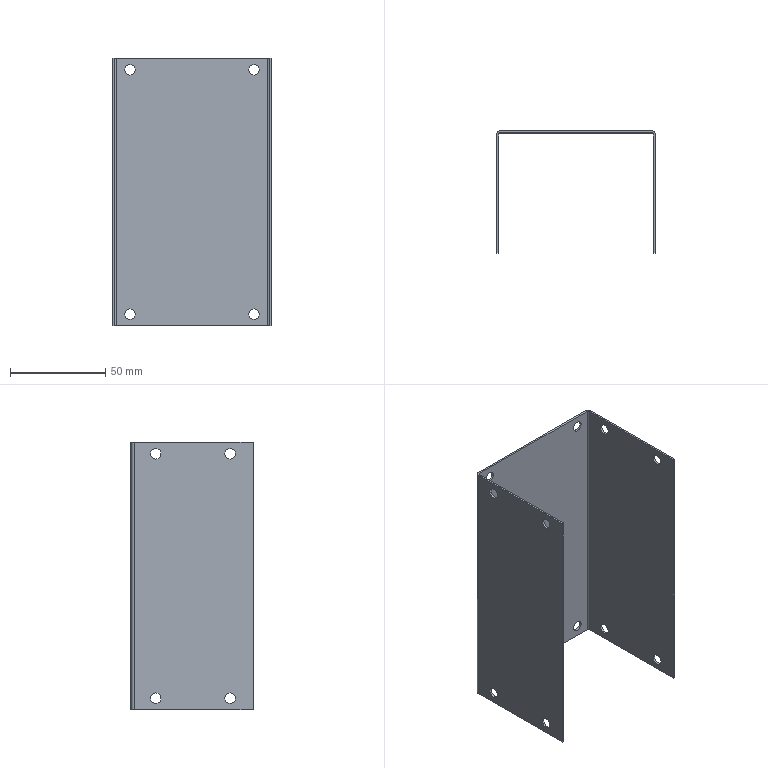Part | SolidWorks | features HoleWzd 2, FlatPattern 1, SMBaseFlange 1, SheetMetal 1 | 1 solid | 46 faces | box 83 x 64 x 140 mm | volume 28826 mm3 | cylinder 28 | plane 18 | commonest cylinder face diameters 5.5 x24 1.473 x2 3.473 x2
STEP:
#1=CARTESIAN_POINT('',(-40.5,51.,136.75));
#2=VERTEX_POINT('',#1);
#3=CARTESIAN_POINT('',(-40.5,51.,131.25));
#4=VERTEX_POINT('',#3);
#5=CARTESIAN_POINT('',(-40.5,51.,134.));
#6=DIRECTION('',(1.,0.,0.));
#7=DIRECTION('',(0.,1.,0.));
#8=AXIS2_PLACEMENT_3D('',#5,#6,#7);
#9=CIRCLE('',#8,2.75);
#10=EDGE_CURVE('',#2,#4,#9,.T.);
#11=ORIENTED_EDGE('',*,*,#10,.T.);
#12=CARTESIAN_POINT('',(-41.5,51.,131.25));
#13=VERTEX_POINT('',#12);
#14=CARTESIAN_POINT('',(-41.5,51.,131.25));
#15=DIRECTION('',(-1.,0.,0.));
#16=VECTOR('',#15,1000.);
#17=LINE('',#14,#16);
#18=EDGE_CURVE('',#4,#13,#17,.T.);
#19=ORIENTED_EDGE('',*,*,#18,.T.);
#20=CARTESIAN_POINT('',(-41.5,51.,136.75));
#21=VERTEX_POINT('',#20);
#22=CARTESIAN_POINT('',(-41.5,51.,134.));
#23=DIRECTION('',(-1.,0.,0.));
#24=DIRECTION('',(0.,0.,1.));
#25=AXIS2_PLACEMENT_3D('',#22,#23,#24);
#26=CIRCLE('',#25,2.75);
#27=EDGE_CURVE('',#13,#21,#26,.T.);
#28=ORIENTED_EDGE('',*,*,#27,.T.);
#29=CARTESIAN_POINT('',(-41.5,51.,136.75));
#30=DIRECTION('',(-1.,0.,0.));
#31=VECTOR('',#30,1000.);
#32=LINE('',#29,#31);
#33=EDGE_CURVE('',#2,#21,#32,.T.);
#34=ORIENTED_EDGE('',*,*,#33,.F.);
#35=EDGE_LOOP('',(#11,#19,#28,#34));
#36=FACE_OUTER_BOUND('',#35,.T.);
#37=CARTESIAN_POINT('',(-41.5,51.,134.));
#38=DIRECTION('',(-1.,0.,0.));
#39=DIRECTION('',(0.,0.,1.));
#40=AXIS2_PLACEMENT_3D('',#37,#38,#39);
#41=CYLINDRICAL_SURFACE('',#40,2.75);
#42=ADVANCED_FACE('',(#36),#41,.F.);
#43=CARTESIAN_POINT('',(41.5,51.,131.25));
#44=VERTEX_POINT('',#43);
#45=CARTESIAN_POINT('',(41.5,51.,136.75));
#46=VERTEX_POINT('',#45);
#47=CARTESIAN_POINT('',(41.5,51.,134.));
#48=DIRECTION('',(-1.,0.,0.));
#49=DIRECTION('',(0.,0.,1.));
#50=AXIS2_PLACEMENT_3D('',#47,#48,#49);
#51=CIRCLE('',#50,2.75);
#52=EDGE_CURVE('',#44,#46,#51,.T.);
#53=ORIENTED_EDGE('',*,*,#52,.F.);
#54=CARTESIAN_POINT('',(40.5,51.,131.25));
#55=VERTEX_POINT('',#54);
#56=CARTESIAN_POINT('',(-41.5,51.,131.25));
#57=DIRECTION('',(-1.,0.,0.));
#58=VECTOR('',#57,1000.);
#59=LINE('',#56,#58);
#60=EDGE_CURVE('',#44,#55,#59,.T.);
#61=ORIENTED_EDGE('',*,*,#60,.T.);
#62=CARTESIAN_POINT('',(40.5,51.,136.75));
#63=VERTEX_POINT('',#62);
#64=CARTESIAN_POINT('',(40.5,51.,134.));
#65=DIRECTION('',(-1.,0.,0.));
#66=DIRECTION('',(0.,-1.,0.));
#67=AXIS2_PLACEMENT_3D('',#64,#65,#66);
#68=CIRCLE('',#67,2.75);
#69=EDGE_CURVE('',#55,#63,#68,.T.);
#70=ORIENTED_EDGE('',*,*,#69,.T.);
#71=CARTESIAN_POINT('',(-41.5,51.,136.75));
#72=DIRECTION('',(-1.,0.,0.));
#73=VECTOR('',#72,1000.);
#74=LINE('',#71,#73);
#75=EDGE_CURVE('',#46,#63,#74,.T.);
#76=ORIENTED_EDGE('',*,*,#75,.F.);
#77=EDGE_LOOP('',(#53,#61,#70,#76));
#78=FACE_OUTER_BOUND('',#77,.T.);
#79=CARTESIAN_POINT('',(-41.5,51.,134.));
#80=DIRECTION('',(-1.,0.,0.));
#81=DIRECTION('',(0.,0.,1.));
#82=AXIS2_PLACEMENT_3D('',#79,#80,#81);
#83=CYLINDRICAL_SURFACE('',#82,2.75);
#84=ADVANCED_FACE('',(#78),#83,.F.);
#85=CARTESIAN_POINT('',(-40.5,12.,136.75));
#86=VERTEX_POINT('',#85);
#87=CARTESIAN_POINT('',(-40.5,12.,131.25));
#88=VERTEX_POINT('',#87);
#89=CARTESIAN_POINT('',(-40.5,12.,134.));
#90=DIRECTION('',(1.,0.,0.));
#91=DIRECTION('',(0.,1.,0.));
#92=AXIS2_PLACEMENT_3D('',#89,#90,#91);
#93=CIRCLE('',#92,2.75);
#94=EDGE_CURVE('',#86,#88,#93,.T.);
#95=ORIENTED_EDGE('',*,*,#94,.T.);
#96=CARTESIAN_POINT('',(-41.5,12.,131.25));
#97=VERTEX_POINT('',#96);
#98=CARTESIAN_POINT('',(-41.5,12.,131.25));
#99=DIRECTION('',(-1.,0.,0.));
#100=VECTOR('',#99,1000.);
#101=LINE('',#98,#100);
#102=EDGE_CURVE('',#88,#97,#101,.T.);
#103=ORIENTED_EDGE('',*,*,#102,.T.);
#104=CARTESIAN_POINT('',(-41.5,12.,136.75));
#105=VERTEX_POINT('',#104);
#106=CARTESIAN_POINT('',(-41.5,12.,134.));
#107=DIRECTION('',(-1.,0.,0.));
#108=DIRECTION('',(0.,0.,1.));
#109=AXIS2_PLACEMENT_3D('',#106,#107,#108);
#110=CIRCLE('',#109,2.75);
#111=EDGE_CURVE('',#97,#105,#110,.T.);
#112=ORIENTED_EDGE('',*,*,#111,.T.);
#113=CARTESIAN_POINT('',(-41.5,12.,136.75));
#114=DIRECTION('',(-1.,0.,0.));
#115=VECTOR('',#114,1000.);
#116=LINE('',#113,#115);
#117=EDGE_CURVE('',#86,#105,#116,.T.);
#118=ORIENTED_EDGE('',*,*,#117,.F.);
#119=EDGE_LOOP('',(#95,#103,#112,#118));
#120=FACE_OUTER_BOUND('',#119,.T.);
#121=CARTESIAN_POINT('',(-41.5,12.,134.));
#122=DIRECTION('',(-1.,0.,0.));
#123=DIRECTION('',(0.,0.,1.));
#124=AXIS2_PLACEMENT_3D('',#121,#122,#123);
#125=CYLINDRICAL_SURFACE('',#124,2.75);
#126=ADVANCED_FACE('',(#120),#125,.F.);
#127=CARTESIAN_POINT('',(41.5,12.,131.25));
#128=VERTEX_POINT('',#127);
#129=CARTESIAN_POINT('',(41.5,12.,136.75));
#130=VERTEX_POINT('',#129);
#131=CARTESIAN_POINT('',(41.5,12.,134.));
#132=DIRECTION('',(-1.,0.,0.));
#133=DIRECTION('',(0.,0.,1.));
#134=AXIS2_PLACEMENT_3D('',#131,#132,#133);
#135=CIRCLE('',#134,2.75);
#136=EDGE_CURVE('',#128,#130,#135,.T.);
#137=ORIENTED_EDGE('',*,*,#136,.F.);
#138=CARTESIAN_POINT('',(40.5,12.,131.25));
#139=VERTEX_POINT('',#138);
#140=CARTESIAN_POINT('',(-41.5,12.,131.25));
#141=DIRECTION('',(-1.,0.,0.));
#142=VECTOR('',#141,1000.);
#143=LINE('',#140,#142);
#144=EDGE_CURVE('',#128,#139,#143,.T.);
#145=ORIENTED_EDGE('',*,*,#144,.T.);
#146=CARTESIAN_POINT('',(40.5,12.,136.75));
#147=VERTEX_POINT('',#146);
#148=CARTESIAN_POINT('',(40.5,12.,134.));
#149=DIRECTION('',(-1.,0.,0.));
#150=DIRECTION('',(0.,-1.,0.));
#151=AXIS2_PLACEMENT_3D('',#148,#149,#150);
#152=CIRCLE('',#151,2.75);
#153=EDGE_CURVE('',#139,#147,#152,.T.);
#154=ORIENTED_EDGE('',*,*,#153,.T.);
#155=CARTESIAN_POINT('',(-41.5,12.,136.75));
#156=DIRECTION('',(-1.,0.,0.));
#157=VECTOR('',#156,1000.);
#158=LINE('',#155,#157);
#159=EDGE_CURVE('',#130,#147,#158,.T.);
#160=ORIENTED_EDGE('',*,*,#159,.F.);
#161=EDGE_LOOP('',(#137,#145,#154,#160));
#162=FACE_OUTER_BOUND('',#161,.T.);
#163=CARTESIAN_POINT('',(-41.5,12.,134.));
#164=DIRECTION('',(-1.,0.,0.));
#165=DIRECTION('',(0.,0.,1.));
#166=AXIS2_PLACEMENT_3D('',#163,#164,#165);
#167=CYLINDRICAL_SURFACE('',#166,2.75);
#168=ADVANCED_FACE('',(#162),#167,.F.);
#169=CARTESIAN_POINT('',(-40.5,51.,8.75));
#170=VERTEX_POINT('',#169);
#171=CARTESIAN_POINT('',(-40.5,51.,3.25));
#172=VERTEX_POINT('',#171);
#173=CARTESIAN_POINT('',(-40.5,51.,6.));
#174=DIRECTION('',(1.,0.,0.));
#175=DIRECTION('',(0.,1.,0.));
#176=AXIS2_PLACEMENT_3D('',#173,#174,#175);
#177=CIRCLE('',#176,2.75);
#178=EDGE_CURVE('',#170,#172,#177,.T.);
#179=ORIENTED_EDGE('',*,*,#178,.T.);
#180=CARTESIAN_POINT('',(-41.5,51.,3.25));
#181=VERTEX_POINT('',#180);
#182=CARTESIAN_POINT('',(-41.5,51.,3.25));
#183=DIRECTION('',(-1.,0.,0.));
#184=VECTOR('',#183,1000.);
#185=LINE('',#182,#184);
#186=EDGE_CURVE('',#172,#181,#185,.T.);
#187=ORIENTED_EDGE('',*,*,#186,.T.);
#188=CARTESIAN_POINT('',(-41.5,51.,8.75));
#189=VERTEX_POINT('',#188);
#190=CARTESIAN_POINT('',(-41.5,51.,6.));
#191=DIRECTION('',(-1.,0.,0.));
#192=DIRECTION('',(0.,0.,1.));
#193=AXIS2_PLACEMENT_3D('',#190,#191,#192);
#194=CIRCLE('',#193,2.75);
#195=EDGE_CURVE('',#181,#189,#194,.T.);
#196=ORIENTED_EDGE('',*,*,#195,.T.);
#197=CARTESIAN_POINT('',(-41.5,51.,8.75));
#198=DIRECTION('',(-1.,0.,0.));
#199=VECTOR('',#198,1000.);
#200=LINE('',#197,#199);
#201=EDGE_CURVE('',#170,#189,#200,.T.);
#202=ORIENTED_EDGE('',*,*,#201,.F.);
#203=EDGE_LOOP('',(#179,#187,#196,#202));
#204=FACE_OUTER_BOUND('',#203,.T.);
#205=CARTESIAN_POINT('',(-41.5,51.,6.));
#206=DIRECTION('',(-1.,0.,0.));
#207=DIRECTION('',(0.,0.,1.));
#208=AXIS2_PLACEMENT_3D('',#205,#206,#207);
#209=CYLINDRICAL_SURFACE('',#208,2.75);
#210=ADVANCED_FACE('',(#204),#209,.F.);
#211=CARTESIAN_POINT('',(41.5,51.,3.25));
#212=VERTEX_POINT('',#211);
#213=CARTESIAN_POINT('',(41.5,51.,8.75));
#214=VERTEX_POINT('',#213);
#215=CARTESIAN_POINT('',(41.5,51.,6.));
#216=DIRECTION('',(-1.,0.,0.));
#217=DIRECTION('',(0.,0.,1.));
#218=AXIS2_PLACEMENT_3D('',#215,#216,#217);
#219=CIRCLE('',#218,2.75);
#220=EDGE_CURVE('',#212,#214,#219,.T.);
#221=ORIENTED_EDGE('',*,*,#220,.F.);
#222=CARTESIAN_POINT('',(40.5,51.,3.25));
#223=VERTEX_POINT('',#222);
#224=CARTESIAN_POINT('',(-41.5,51.,3.25));
#225=DIRECTION('',(-1.,0.,0.));
#226=VECTOR('',#225,1000.);
#227=LINE('',#224,#226);
#228=EDGE_CURVE('',#212,#223,#227,.T.);
#229=ORIENTED_EDGE('',*,*,#228,.T.);
#230=CARTESIAN_POINT('',(40.5,51.,8.75));
#231=VERTEX_POINT('',#230);
#232=CARTESIAN_POINT('',(40.5,51.,6.));
#233=DIRECTION('',(-1.,0.,0.));
#234=DIRECTION('',(0.,-1.,0.));
#235=AXIS2_PLACEMENT_3D('',#232,#233,#234);
#236=CIRCLE('',#235,2.75);
#237=EDGE_CURVE('',#223,#231,#236,.T.);
#238=ORIENTED_EDGE('',*,*,#237,.T.);
#239=CARTESIAN_POINT('',(-41.5,51.,8.75));
#240=DIRECTION('',(-1.,0.,0.));
#241=VECTOR('',#240,1000.);
#242=LINE('',#239,#241);
#243=EDGE_CURVE('',#214,#231,#242,.T.);
#244=ORIENTED_EDGE('',*,*,#243,.F.);
#245=EDGE_LOOP('',(#221,#229,#238,#244));
#246=FACE_OUTER_BOUND('',#245,.T.);
#247=CARTESIAN_POINT('',(-41.5,51.,6.));
#248=DIRECTION('',(-1.,0.,0.));
#249=DIRECTION('',(0.,0.,1.));
#250=AXIS2_PLACEMENT_3D('',#247,#248,#249);
#251=CYLINDRICAL_SURFACE('',#250,2.75);
#252=ADVANCED_FACE('',(#246),#251,.F.);
#253=CARTESIAN_POINT('',(-40.5,12.,8.75));
#254=VERTEX_POINT('',#253);
#255=CARTESIAN_POINT('',(-40.5,12.,3.25));
#256=VERTEX_POINT('',#255);
#257=CARTESIAN_POINT('',(-40.5,12.,6.));
#258=DIRECTION('',(1.,0.,0.));
#259=DIRECTION('',(0.,1.,0.));
#260=AXIS2_PLACEMENT_3D('',#257,#258,#259);
#261=CIRCLE('',#260,2.75);
#262=EDGE_CURVE('',#254,#256,#261,.T.);
#263=ORIENTED_EDGE('',*,*,#262,.T.);
#264=CARTESIAN_POINT('',(-41.5,12.,3.25));
#265=VERTEX_POINT('',#264);
#266=CARTESIAN_POINT('',(-41.5,12.,3.25));
#267=DIRECTION('',(-1.,0.,0.));
#268=VECTOR('',#267,1000.);
#269=LINE('',#266,#268);
#270=EDGE_CURVE('',#256,#265,#269,.T.);
#271=ORIENTED_EDGE('',*,*,#270,.T.);
#272=CARTESIAN_POINT('',(-41.5,12.,8.75));
#273=VERTEX_POINT('',#272);
#274=CARTESIAN_POINT('',(-41.5,12.,6.));
#275=DIRECTION('',(-1.,0.,0.));
#276=DIRECTION('',(0.,0.,1.));
#277=AXIS2_PLACEMENT_3D('',#274,#275,#276);
#278=CIRCLE('',#277,2.75);
#279=EDGE_CURVE('',#265,#273,#278,.T.);
#280=ORIENTED_EDGE('',*,*,#279,.T.);
#281=CARTESIAN_POINT('',(-41.5,12.,8.75));
#282=DIRECTION('',(-1.,0.,0.));
#283=VECTOR('',#282,1000.);
#284=LINE('',#281,#283);
#285=EDGE_CURVE('',#254,#273,#284,.T.);
#286=ORIENTED_EDGE('',*,*,#285,.F.);
#287=EDGE_LOOP('',(#263,#271,#280,#286));
#288=FACE_OUTER_BOUND('',#287,.T.);
#289=CARTESIAN_POINT('',(-41.5,12.,6.));
#290=DIRECTION('',(-1.,0.,0.));
#291=DIRECTION('',(0.,0.,1.));
#292=AXIS2_PLACEMENT_3D('',#289,#290,#291);
#293=CYLINDRICAL_SURFACE('',#292,2.75);
#294=ADVANCED_FACE('',(#288),#293,.F.);
#295=CARTESIAN_POINT('',(41.5,12.,3.25));
#296=VERTEX_POINT('',#295);
#297=CARTESIAN_POINT('',(41.5,12.,8.75));
#298=VERTEX_POINT('',#297);
#299=CARTESIAN_POINT('',(41.5,12.,6.));
#300=DIRECTION('',(-1.,0.,0.));
#301=DIRECTION('',(0.,0.,1.));
#302=AXIS2_PLACEMENT_3D('',#299,#300,#301);
#303=CIRCLE('',#302,2.75);
#304=EDGE_CURVE('',#296,#298,#303,.T.);
#305=ORIENTED_EDGE('',*,*,#304,.F.);
#306=CARTESIAN_POINT('',(40.5,12.,3.25));
#307=VERTEX_POINT('',#306);
#308=CARTESIAN_POINT('',(-41.5,12.,3.25));
#309=DIRECTION('',(-1.,0.,0.));
#310=VECTOR('',#309,1000.);
#311=LINE('',#308,#310);
#312=EDGE_CURVE('',#296,#307,#311,.T.);
#313=ORIENTED_EDGE('',*,*,#312,.T.);
#314=CARTESIAN_POINT('',(40.5,12.,8.75));
#315=VERTEX_POINT('',#314);
#316=CARTESIAN_POINT('',(40.5,12.,6.));
#317=DIRECTION('',(-1.,0.,0.));
#318=DIRECTION('',(0.,-1.,0.));
#319=AXIS2_PLACEMENT_3D('',#316,#317,#318);
#320=CIRCLE('',#319,2.75);
#321=EDGE_CURVE('',#307,#315,#320,.T.);
#322=ORIENTED_EDGE('',*,*,#321,.T.);
#323=CARTESIAN_POINT('',(-41.5,12.,8.75));
#324=DIRECTION('',(-1.,0.,0.));
#325=VECTOR('',#324,1000.);
#326=LINE('',#323,#325);
#327=EDGE_CURVE('',#298,#315,#326,.T.);
#328=ORIENTED_EDGE('',*,*,#327,.F.);
#329=EDGE_LOOP('',(#305,#313,#322,#328));
#330=FACE_OUTER_BOUND('',#329,.T.);
#331=CARTESIAN_POINT('',(-41.5,12.,6.));
#332=DIRECTION('',(-1.,0.,0.));
#333=DIRECTION('',(0.,0.,1.));
#334=AXIS2_PLACEMENT_3D('',#331,#332,#333);
#335=CYLINDRICAL_SURFACE('',#334,2.75);
#336=ADVANCED_FACE('',(#330),#335,.F.);
#337=CARTESIAN_POINT('',(-32.5,63.,8.75));
#338=VERTEX_POINT('',#337);
#339=CARTESIAN_POINT('',(-32.5,63.,3.25));
#340=VERTEX_POINT('',#339);
#341=CARTESIAN_POINT('',(-32.5,63.,6.));
#342=DIRECTION('',(0.,-1.,0.));
#343=DIRECTION('',(0.,0.,-1.));
#344=AXIS2_PLACEMENT_3D('',#341,#342,#343);
#345=CIRCLE('',#344,2.75);
#346=EDGE_CURVE('',#338,#340,#345,.T.);
#347=ORIENTED_EDGE('',*,*,#346,.T.);
#348=CARTESIAN_POINT('',(-32.5,64.,3.25));
#349=VERTEX_POINT('',#348);
#350=CARTESIAN_POINT('',(-32.5,64.,3.25));
#351=DIRECTION('',(0.,1.,0.));
#352=VECTOR('',#351,1000.);
#353=LINE('',#350,#352);
#354=EDGE_CURVE('',#340,#349,#353,.T.);
#355=ORIENTED_EDGE('',*,*,#354,.T.);
#356=CARTESIAN_POINT('',(-32.5,64.,8.75));
#357=VERTEX_POINT('',#356);
#358=CARTESIAN_POINT('',(-32.5,64.,6.));
#359=DIRECTION('',(0.,1.,0.));
#360=DIRECTION('',(0.,0.,1.));
#361=AXIS2_PLACEMENT_3D('',#358,#359,#360);
#362=CIRCLE('',#361,2.75);
#363=EDGE_CURVE('',#349,#357,#362,.T.);
#364=ORIENTED_EDGE('',*,*,#363,.T.);
#365=CARTESIAN_POINT('',(-32.5,64.,8.75));
#366=DIRECTION('',(0.,1.,0.));
#367=VECTOR('',#366,1000.);
#368=LINE('',#365,#367);
#369=EDGE_CURVE('',#338,#357,#368,.T.);
#370=ORIENTED_EDGE('',*,*,#369,.F.);
#371=EDGE_LOOP('',(#347,#355,#364,#370));
#372=FACE_OUTER_BOUND('',#371,.T.);
#373=CARTESIAN_POINT('',(-32.5,64.,6.));
#374=DIRECTION('',(0.,1.,0.));
#375=DIRECTION('',(0.,0.,1.));
#376=AXIS2_PLACEMENT_3D('',#373,#374,#375);
#377=CYLINDRICAL_SURFACE('',#376,2.75);
#378=ADVANCED_FACE('',(#372),#377,.F.);
#379=CARTESIAN_POINT('',(32.5,63.,8.75));
#380=VERTEX_POINT('',#379);
#381=CARTESIAN_POINT('',(32.5,63.,3.25));
#382=VERTEX_POINT('',#381);
#383=CARTESIAN_POINT('',(32.5,63.,6.));
#384=DIRECTION('',(0.,-1.,0.));
#385=DIRECTION('',(0.,0.,-1.));
#386=AXIS2_PLACEMENT_3D('',#383,#384,#385);
#387=CIRCLE('',#386,2.75);
#388=EDGE_CURVE('',#380,#382,#387,.T.);
#389=ORIENTED_EDGE('',*,*,#388,.T.);
#390=CARTESIAN_POINT('',(32.5,64.,3.25));
#391=VERTEX_POINT('',#390);
#392=CARTESIAN_POINT('',(32.5,64.,3.25));
#393=DIRECTION('',(0.,1.,0.));
#394=VECTOR('',#393,1000.);
#395=LINE('',#392,#394);
#396=EDGE_CURVE('',#382,#391,#395,.T.);
#397=ORIENTED_EDGE('',*,*,#396,.T.);
#398=CARTESIAN_POINT('',(32.5,64.,8.75));
#399=VERTEX_POINT('',#398);
#400=CARTESIAN_POINT('',(32.5,64.,6.));
#401=DIRECTION('',(0.,1.,0.));
#402=DIRECTION('',(0.,0.,1.));
#403=AXIS2_PLACEMENT_3D('',#400,#401,#402);
#404=CIRCLE('',#403,2.75);
#405=EDGE_CURVE('',#391,#399,#404,.T.);
#406=ORIENTED_EDGE('',*,*,#405,.T.);
#407=CARTESIAN_POINT('',(32.5,64.,8.75));
#408=DIRECTION('',(0.,1.,0.));
#409=VECTOR('',#408,1000.);
#410=LINE('',#407,#409);
#411=EDGE_CURVE('',#380,#399,#410,.T.);
#412=ORIENTED_EDGE('',*,*,#411,.F.);
#413=EDGE_LOOP('',(#389,#397,#406,#412));
#414=FACE_OUTER_BOUND('',#413,.T.);
#415=CARTESIAN_POINT('',(32.5,64.,6.));
#416=DIRECTION('',(0.,1.,0.));
#417=DIRECTION('',(0.,0.,1.));
#418=AXIS2_PLACEMENT_3D('',#415,#416,#417);
#419=CYLINDRICAL_SURFACE('',#418,2.75);
#420=ADVANCED_FACE('',(#414),#419,.F.);
#421=CARTESIAN_POINT('',(32.5,63.,136.75));
#422=VERTEX_POINT('',#421);
#423=CARTESIAN_POINT('',(32.5,63.,131.25));
#424=VERTEX_POINT('',#423);
#425=CARTESIAN_POINT('',(32.5,63.,134.));
#426=DIRECTION('',(0.,-1.,0.));
#427=DIRECTION('',(0.,0.,-1.));
#428=AXIS2_PLACEMENT_3D('',#425,#426,#427);
#429=CIRCLE('',#428,2.75);
#430=EDGE_CURVE('',#422,#424,#429,.T.);
#431=ORIENTED_EDGE('',*,*,#430,.T.);
#432=CARTESIAN_POINT('',(32.5,64.,131.25));
#433=VERTEX_POINT('',#432);
#434=CARTESIAN_POINT('',(32.5,64.,131.25));
#435=DIRECTION('',(0.,1.,0.));
#436=VECTOR('',#435,1000.);
#437=LINE('',#434,#436);
#438=EDGE_CURVE('',#424,#433,#437,.T.);
#439=ORIENTED_EDGE('',*,*,#438,.T.);
#440=CARTESIAN_POINT('',(32.5,64.,136.75));
#441=VERTEX_POINT('',#440);
#442=CARTESIAN_POINT('',(32.5,64.,134.));
#443=DIRECTION('',(0.,1.,0.));
#444=DIRECTION('',(0.,0.,1.));
#445=AXIS2_PLACEMENT_3D('',#442,#443,#444);
#446=CIRCLE('',#445,2.75);
#447=EDGE_CURVE('',#433,#441,#446,.T.);
#448=ORIENTED_EDGE('',*,*,#447,.T.);
#449=CARTESIAN_POINT('',(32.5,64.,136.75));
#450=DIRECTION('',(0.,1.,0.));
#451=VECTOR('',#450,1000.);
#452=LINE('',#449,#451);
#453=EDGE_CURVE('',#422,#441,#452,.T.);
#454=ORIENTED_EDGE('',*,*,#453,.F.);
#455=EDGE_LOOP('',(#431,#439,#448,#454));
#456=FACE_OUTER_BOUND('',#455,.T.);
#457=CARTESIAN_POINT('',(32.5,64.,134.));
#458=DIRECTION('',(0.,1.,0.));
#459=DIRECTION('',(0.,0.,1.));
#460=AXIS2_PLACEMENT_3D('',#457,#458,#459);
#461=CYLINDRICAL_SURFACE('',#460,2.75);
#462=ADVANCED_FACE('',(#456),#461,.F.);
#463=CARTESIAN_POINT('',(-32.5,63.,136.75));
#464=VERTEX_POINT('',#463);
#465=CARTESIAN_POINT('',(-32.5,63.,131.25));
#466=VERTEX_POINT('',#465);
#467=CARTESIAN_POINT('',(-32.5,63.,134.));
#468=DIRECTION('',(0.,-1.,0.));
#469=DIRECTION('',(0.,0.,-1.));
#470=AXIS2_PLACEMENT_3D('',#467,#468,#469);
#471=CIRCLE('',#470,2.75);
#472=EDGE_CURVE('',#464,#466,#471,.T.);
#473=ORIENTED_EDGE('',*,*,#472,.T.);
#474=CARTESIAN_POINT('',(-32.5,64.,131.25));
#475=VERTEX_POINT('',#474);
#476=CARTESIAN_POINT('',(-32.5,64.,131.25));
#477=DIRECTION('',(0.,1.,0.));
#478=VECTOR('',#477,1000.);
#479=LINE('',#476,#478);
#480=EDGE_CURVE('',#466,#475,#479,.T.);
#481=ORIENTED_EDGE('',*,*,#480,.T.);
#482=CARTESIAN_POINT('',(-32.5,64.,136.75));
#483=VERTEX_POINT('',#482);
#484=CARTESIAN_POINT('',(-32.5,64.,134.));
#485=DIRECTION('',(0.,1.,0.));
#486=DIRECTION('',(0.,0.,1.));
#487=AXIS2_PLACEMENT_3D('',#484,#485,#486);
#488=CIRCLE('',#487,2.75);
#489=EDGE_CURVE('',#475,#483,#488,.T.);
#490=ORIENTED_EDGE('',*,*,#489,.T.);
#491=CARTESIAN_POINT('',(-32.5,64.,136.75));
#492=DIRECTION('',(0.,1.,0.));
#493=VECTOR('',#492,1000.);
#494=LINE('',#491,#493);
#495=EDGE_CURVE('',#464,#483,#494,.T.);
#496=ORIENTED_EDGE('',*,*,#495,.F.);
#497=EDGE_LOOP('',(#473,#481,#490,#496));
#498=FACE_OUTER_BOUND('',#497,.T.);
#499=CARTESIAN_POINT('',(-32.5,64.,134.));
#500=DIRECTION('',(0.,1.,0.));
#501=DIRECTION('',(0.,0.,1.));
#502=AXIS2_PLACEMENT_3D('',#499,#500,#501);
#503=CYLINDRICAL_SURFACE('',#502,2.75);
#504=ADVANCED_FACE('',(#498),#503,.F.);
#505=CARTESIAN_POINT('',(-32.5,64.,6.));
#506=DIRECTION('',(0.,1.,0.));
#507=DIRECTION('',(0.,0.,1.));
#508=AXIS2_PLACEMENT_3D('',#505,#506,#507);
#509=CIRCLE('',#508,2.75);
#510=EDGE_CURVE('',#357,#349,#509,.T.);
#511=ORIENTED_EDGE('',*,*,#510,.F.);
#512=ORIENTED_EDGE('',*,*,#363,.F.);
#513=EDGE_LOOP('',(#511,#512));
#514=FACE_BOUND('',#513,.T.);
#515=CARTESIAN_POINT('',(32.5,64.,134.));
#516=DIRECTION('',(0.,1.,0.));
#517=DIRECTION('',(0.,0.,1.));
#518=AXIS2_PLACEMENT_3D('',#515,#516,#517);
#519=CIRCLE('',#518,2.75);
#520=EDGE_CURVE('',#441,#433,#519,.T.);
#521=ORIENTED_EDGE('',*,*,#520,.F.);
#522=ORIENTED_EDGE('',*,*,#447,.F.);
#523=EDGE_LOOP('',(#521,#522));
#524=FACE_BOUND('',#523,.T.);
#525=CARTESIAN_POINT('',(-32.5,64.,134.));
#526=DIRECTION('',(0.,1.,0.));
#527=DIRECTION('',(0.,0.,1.));
#528=AXIS2_PLACEMENT_3D('',#525,#526,#527);
#529=CIRCLE('',#528,2.75);
#530=EDGE_CURVE('',#483,#475,#529,.T.);
#531=ORIENTED_EDGE('',*,*,#530,.F.);
#532=ORIENTED_EDGE('',*,*,#489,.F.);
#533=EDGE_LOOP('',(#531,#532));
#534=FACE_BOUND('',#533,.T.);
#535=CARTESIAN_POINT('',(39.763,64.,0.));
#536=VERTEX_POINT('',#535);
#537=CARTESIAN_POINT('',(-39.763,64.,0.));
#538=VERTEX_POINT('',#537);
#539=CARTESIAN_POINT('',(-40.5,64.,0.));
#540=DIRECTION('',(-1.,0.,0.));
#541=VECTOR('',#540,1000.);
#542=LINE('',#539,#541);
#543=EDGE_CURVE('',#536,#538,#542,.T.);
#544=ORIENTED_EDGE('',*,*,#543,.T.);
#545=CARTESIAN_POINT('',(-39.763,64.,140.));
#546=VERTEX_POINT('',#545);
#547=CARTESIAN_POINT('',(-39.763,64.,140.));
#548=DIRECTION('',(0.,0.,-1.));
#549=VECTOR('',#548,1000.);
#550=LINE('',#547,#549);
#551=EDGE_CURVE('',#546,#538,#550,.T.);
#552=ORIENTED_EDGE('',*,*,#551,.F.);
#553=CARTESIAN_POINT('',(39.763,64.,140.));
#554=VERTEX_POINT('',#553);
#555=CARTESIAN_POINT('',(-40.5,64.,140.));
#556=DIRECTION('',(-1.,0.,0.));
#557=VECTOR('',#556,1000.);
#558=LINE('',#555,#557);
#559=EDGE_CURVE('',#554,#546,#558,.T.);
#560=ORIENTED_EDGE('',*,*,#559,.F.);
#561=CARTESIAN_POINT('',(39.763,64.,140.));
#562=DIRECTION('',(0.,0.,-1.));
#563=VECTOR('',#562,1000.);
#564=LINE('',#561,#563);
#565=EDGE_CURVE('',#554,#536,#564,.T.);
#566=ORIENTED_EDGE('',*,*,#565,.T.);
#567=EDGE_LOOP('',(#544,#552,#560,#566));
#568=FACE_OUTER_BOUND('',#567,.T.);
#569=CARTESIAN_POINT('',(32.5,64.,6.));
#570=DIRECTION('',(0.,1.,0.));
#571=DIRECTION('',(0.,0.,1.));
#572=AXIS2_PLACEMENT_3D('',#569,#570,#571);
#573=CIRCLE('',#572,2.75);
#574=EDGE_CURVE('',#399,#391,#573,.T.);
#575=ORIENTED_EDGE('',*,*,#574,.F.);
#576=ORIENTED_EDGE('',*,*,#405,.F.);
#577=EDGE_LOOP('',(#575,#576));
#578=FACE_BOUND('',#577,.T.);
#579=CARTESIAN_POINT('',(-40.5,64.,140.));
#580=DIRECTION('',(0.,-1.,0.));
#581=DIRECTION('',(0.,0.,-1.));
#582=AXIS2_PLACEMENT_3D('',#579,#580,#581);
#583=PLANE('',#582);
#584=ADVANCED_FACE('',(#514,#524,#534,#568,#578),#583,.F.);
#585=CARTESIAN_POINT('',(39.763,63.,140.));
#586=VERTEX_POINT('',#585);
#587=CARTESIAN_POINT('',(39.763,63.,140.));
#588=DIRECTION('',(0.,1.,0.));
#589=VECTOR('',#588,1000.);
#590=LINE('',#587,#589);
#591=EDGE_CURVE('',#586,#554,#590,.T.);
#592=ORIENTED_EDGE('',*,*,#591,.F.);
#593=CARTESIAN_POINT('',(40.5,62.263,140.));
#594=VERTEX_POINT('',#593);
#595=CARTESIAN_POINT('',(39.763,62.263,140.));
#596=DIRECTION('',(0.,0.,1.));
#597=DIRECTION('',(-1.,0.,0.));
#598=AXIS2_PLACEMENT_3D('',#595,#596,#597);
#599=CIRCLE('',#598,0.7366);
#600=EDGE_CURVE('',#594,#586,#599,.T.);
#601=ORIENTED_EDGE('',*,*,#600,.F.);
#602=CARTESIAN_POINT('',(41.5,62.263,140.));
#603=VERTEX_POINT('',#602);
#604=CARTESIAN_POINT('',(41.5,62.263,140.));
#605=DIRECTION('',(-1.,0.,0.));
#606=VECTOR('',#605,1000.);
#607=LINE('',#604,#606);
#608=EDGE_CURVE('',#603,#594,#607,.T.);
#609=ORIENTED_EDGE('',*,*,#608,.F.);
#610=CARTESIAN_POINT('',(39.763,62.263,140.));
#611=DIRECTION('',(0.,0.,1.));
#612=DIRECTION('',(1.,0.,0.));
#613=AXIS2_PLACEMENT_3D('',#610,#611,#612);
#614=CIRCLE('',#613,1.737);
#615=EDGE_CURVE('',#603,#554,#614,.T.);
#616=ORIENTED_EDGE('',*,*,#615,.T.);
#617=EDGE_LOOP('',(#592,#601,#609,#616));
#618=FACE_OUTER_BOUND('',#617,.T.);
#619=CARTESIAN_POINT('',(39.763,63.,140.));
#620=DIRECTION('',(0.,0.,1.));
#621=DIRECTION('',(1.,0.,0.));
#622=AXIS2_PLACEMENT_3D('',#619,#620,#621);
#623=PLANE('',#622);
#624=ADVANCED_FACE('',(#618),#623,.T.);
#625=CARTESIAN_POINT('',(-39.763,63.,140.));
#626=VERTEX_POINT('',#625);
#627=CARTESIAN_POINT('',(-40.5,63.,140.));
#628=DIRECTION('',(-1.,0.,0.));
#629=VECTOR('',#628,1000.);
#630=LINE('',#627,#629);
#631=EDGE_CURVE('',#586,#626,#630,.T.);
#632=ORIENTED_EDGE('',*,*,#631,.F.);
#633=ORIENTED_EDGE('',*,*,#591,.T.);
#634=ORIENTED_EDGE('',*,*,#559,.T.);
#635=CARTESIAN_POINT('',(-39.763,64.,140.));
#636=DIRECTION('',(0.,-1.,0.));
#637=VECTOR('',#636,1000.);
#638=LINE('',#635,#637);
#639=EDGE_CURVE('',#546,#626,#638,.T.);
#640=ORIENTED_EDGE('',*,*,#639,.T.);
#641=EDGE_LOOP('',(#632,#633,#634,#640));
#642=FACE_OUTER_BOUND('',#641,.T.);
#643=CARTESIAN_POINT('',(41.5,62.263,140.));
#644=DIRECTION('',(0.,0.,1.));
#645=DIRECTION('',(1.,0.,0.));
#646=AXIS2_PLACEMENT_3D('',#643,#644,#645);
#647=PLANE('',#646);
#648=ADVANCED_FACE('',(#642),#647,.T.);
#649=CARTESIAN_POINT('',(40.5,62.263,0.));
#650=VERTEX_POINT('',#649);
#651=CARTESIAN_POINT('',(41.5,62.263,0.));
#652=VERTEX_POINT('',#651);
#653=CARTESIAN_POINT('',(40.5,62.263,0.));
#654=DIRECTION('',(1.,0.,0.));
#655=VECTOR('',#654,1000.);
#656=LINE('',#653,#655);
#657=EDGE_CURVE('',#650,#652,#656,.T.);
#658=ORIENTED_EDGE('',*,*,#657,.F.);
#659=CARTESIAN_POINT('',(39.763,63.,0.));
#660=VERTEX_POINT('',#659);
#661=CARTESIAN_POINT('',(39.763,62.263,0.));
#662=DIRECTION('',(0.,0.,1.));
#663=DIRECTION('',(-1.,0.,0.));
#664=AXIS2_PLACEMENT_3D('',#661,#662,#663);
#665=CIRCLE('',#664,0.7366);
#666=EDGE_CURVE('',#650,#660,#665,.T.);
#667=ORIENTED_EDGE('',*,*,#666,.T.);
#668=CARTESIAN_POINT('',(39.763,64.,0.));
#669=DIRECTION('',(0.,-1.,0.));
#670=VECTOR('',#669,1000.);
#671=LINE('',#668,#670);
#672=EDGE_CURVE('',#536,#660,#671,.T.);
#673=ORIENTED_EDGE('',*,*,#672,.F.);
#674=CARTESIAN_POINT('',(39.763,62.263,0.));
#675=DIRECTION('',(0.,0.,1.));
#676=DIRECTION('',(1.,0.,0.));
#677=AXIS2_PLACEMENT_3D('',#674,#675,#676);
#678=CIRCLE('',#677,1.737);
#679=EDGE_CURVE('',#652,#536,#678,.T.);
#680=ORIENTED_EDGE('',*,*,#679,.F.);
#681=EDGE_LOOP('',(#658,#667,#673,#680));
#682=FACE_OUTER_BOUND('',#681,.T.);
#683=CARTESIAN_POINT('',(40.5,62.263,0.));
#684=DIRECTION('',(0.,0.,-1.));
#685=DIRECTION('',(-1.,0.,0.));
#686=AXIS2_PLACEMENT_3D('',#683,#684,#685);
#687=PLANE('',#686);
#688=ADVANCED_FACE('',(#682),#687,.T.);
#689=CARTESIAN_POINT('',(40.5,0.,0.));
#690=VERTEX_POINT('',#689);
#691=CARTESIAN_POINT('',(40.5,63.,0.));
#692=DIRECTION('',(0.,1.,0.));
#693=VECTOR('',#692,1000.);
#694=LINE('',#691,#693);
#695=EDGE_CURVE('',#690,#650,#694,.T.);
#696=ORIENTED_EDGE('',*,*,#695,.T.);
#697=ORIENTED_EDGE('',*,*,#657,.T.);
#698=CARTESIAN_POINT('',(41.5,0.,0.));
#699=VERTEX_POINT('',#698);
#700=CARTESIAN_POINT('',(41.5,63.,0.));
#701=DIRECTION('',(0.,1.,0.));
#702=VECTOR('',#701,1000.);
#703=LINE('',#700,#702);
#704=EDGE_CURVE('',#699,#652,#703,.T.);
#705=ORIENTED_EDGE('',*,*,#704,.F.);
#706=CARTESIAN_POINT('',(41.5,0.,0.));
#707=DIRECTION('',(-1.,0.,0.));
#708=VECTOR('',#707,1000.);
#709=LINE('',#706,#708);
#710=EDGE_CURVE('',#699,#690,#709,.T.);
#711=ORIENTED_EDGE('',*,*,#710,.T.);
#712=EDGE_LOOP('',(#696,#697,#705,#711));
#713=FACE_OUTER_BOUND('',#712,.T.);
#714=CARTESIAN_POINT('',(39.763,64.,0.));
#715=DIRECTION('',(0.,0.,-1.));
#716=DIRECTION('',(-1.,0.,0.));
#717=AXIS2_PLACEMENT_3D('',#714,#715,#716);
#718=PLANE('',#717);
#719=ADVANCED_FACE('',(#713),#718,.T.);
#720=CARTESIAN_POINT('',(-40.5,62.263,140.));
#721=VERTEX_POINT('',#720);
#722=CARTESIAN_POINT('',(-41.5,62.263,140.));
#723=VERTEX_POINT('',#722);
#724=CARTESIAN_POINT('',(-40.5,62.263,140.));
#725=DIRECTION('',(-1.,0.,0.));
#726=VECTOR('',#725,1000.);
#727=LINE('',#724,#726);
#728=EDGE_CURVE('',#721,#723,#727,.T.);
#729=ORIENTED_EDGE('',*,*,#728,.F.);
#730=CARTESIAN_POINT('',(-39.763,62.263,140.));
#731=DIRECTION('',(0.,0.,1.));
#732=DIRECTION('',(-1.,0.,0.));
#733=AXIS2_PLACEMENT_3D('',#730,#731,#732);
#734=CIRCLE('',#733,0.7366);
#735=EDGE_CURVE('',#626,#721,#734,.T.);
#736=ORIENTED_EDGE('',*,*,#735,.F.);
#737=ORIENTED_EDGE('',*,*,#639,.F.);
#738=CARTESIAN_POINT('',(-39.763,62.263,140.));
#739=DIRECTION('',(0.,0.,1.));
#740=DIRECTION('',(1.,0.,0.));
#741=AXIS2_PLACEMENT_3D('',#738,#739,#740);
#742=CIRCLE('',#741,1.737);
#743=EDGE_CURVE('',#546,#723,#742,.T.);
#744=ORIENTED_EDGE('',*,*,#743,.T.);
#745=EDGE_LOOP('',(#729,#736,#737,#744));
#746=FACE_OUTER_BOUND('',#745,.T.);
#747=CARTESIAN_POINT('',(-40.5,62.263,140.));
#748=DIRECTION('',(0.,0.,1.));
#749=DIRECTION('',(1.,0.,0.));
#750=AXIS2_PLACEMENT_3D('',#747,#748,#749);
#751=PLANE('',#750);
#752=ADVANCED_FACE('',(#746),#751,.T.);
#753=CARTESIAN_POINT('',(-40.5,0.,140.));
#754=VERTEX_POINT('',#753);
#755=CARTESIAN_POINT('',(-40.5,63.,140.));
#756=DIRECTION('',(0.,-1.,0.));
#757=VECTOR('',#756,1000.);
#758=LINE('',#755,#757);
#759=EDGE_CURVE('',#721,#754,#758,.T.);
#760=ORIENTED_EDGE('',*,*,#759,.F.);
#761=ORIENTED_EDGE('',*,*,#728,.T.);
#762=CARTESIAN_POINT('',(-41.5,0.,140.));
#763=VERTEX_POINT('',#762);
#764=CARTESIAN_POINT('',(-41.5,63.,140.));
#765=DIRECTION('',(0.,-1.,0.));
#766=VECTOR('',#765,1000.);
#767=LINE('',#764,#766);
#768=EDGE_CURVE('',#723,#763,#767,.T.);
#769=ORIENTED_EDGE('',*,*,#768,.T.);
#770=CARTESIAN_POINT('',(-40.5,0.,140.));
#771=DIRECTION('',(-1.,0.,0.));
#772=VECTOR('',#771,1000.);
#773=LINE('',#770,#772);
#774=EDGE_CURVE('',#754,#763,#773,.T.);
#775=ORIENTED_EDGE('',*,*,#774,.F.);
#776=EDGE_LOOP('',(#760,#761,#769,#775));
#777=FACE_OUTER_BOUND('',#776,.T.);
#778=CARTESIAN_POINT('',(-39.763,64.,140.));
#779=DIRECTION('',(0.,0.,1.));
#780=DIRECTION('',(1.,0.,0.));
#781=AXIS2_PLACEMENT_3D('',#778,#779,#780);
#782=PLANE('',#781);
#783=ADVANCED_FACE('',(#777),#782,.T.);
#784=CARTESIAN_POINT('',(-39.763,63.,0.));
#785=VERTEX_POINT('',#784);
#786=CARTESIAN_POINT('',(-39.763,63.,0.));
#787=DIRECTION('',(0.,1.,0.));
#788=VECTOR('',#787,1000.);
#789=LINE('',#786,#788);
#790=EDGE_CURVE('',#785,#538,#789,.T.);
#791=ORIENTED_EDGE('',*,*,#790,.F.);
#792=CARTESIAN_POINT('',(-40.5,62.263,0.));
#793=VERTEX_POINT('',#792);
#794=CARTESIAN_POINT('',(-39.763,62.263,0.));
#795=DIRECTION('',(0.,0.,1.));
#796=DIRECTION('',(-1.,0.,0.));
#797=AXIS2_PLACEMENT_3D('',#794,#795,#796);
#798=CIRCLE('',#797,0.7366);
#799=EDGE_CURVE('',#785,#793,#798,.T.);
#800=ORIENTED_EDGE('',*,*,#799,.T.);
#801=CARTESIAN_POINT('',(-41.5,62.263,0.));
#802=VERTEX_POINT('',#801);
#803=CARTESIAN_POINT('',(-41.5,62.263,0.));
#804=DIRECTION('',(1.,0.,0.));
#805=VECTOR('',#804,1000.);
#806=LINE('',#803,#805);
#807=EDGE_CURVE('',#802,#793,#806,.T.);
#808=ORIENTED_EDGE('',*,*,#807,.F.);
#809=CARTESIAN_POINT('',(-39.763,62.263,0.));
#810=DIRECTION('',(0.,0.,1.));
#811=DIRECTION('',(1.,0.,0.));
#812=AXIS2_PLACEMENT_3D('',#809,#810,#811);
#813=CIRCLE('',#812,1.737);
#814=EDGE_CURVE('',#538,#802,#813,.T.);
#815=ORIENTED_EDGE('',*,*,#814,.F.);
#816=EDGE_LOOP('',(#791,#800,#808,#815));
#817=FACE_OUTER_BOUND('',#816,.T.);
#818=CARTESIAN_POINT('',(-39.763,63.,0.));
#819=DIRECTION('',(0.,0.,-1.));
#820=DIRECTION('',(-1.,0.,0.));
#821=AXIS2_PLACEMENT_3D('',#818,#819,#820);
#822=PLANE('',#821);
#823=ADVANCED_FACE('',(#817),#822,.T.);
#824=CARTESIAN_POINT('',(-40.5,63.,0.));
#825=DIRECTION('',(-1.,0.,0.));
#826=VECTOR('',#825,1000.);
#827=LINE('',#824,#826);
#828=EDGE_CURVE('',#660,#785,#827,.T.);
#829=ORIENTED_EDGE('',*,*,#828,.T.);
#830=ORIENTED_EDGE('',*,*,#790,.T.);
#831=ORIENTED_EDGE('',*,*,#543,.F.);
#832=ORIENTED_EDGE('',*,*,#672,.T.);
#833=EDGE_LOOP('',(#829,#830,#831,#832));
#834=FACE_OUTER_BOUND('',#833,.T.);
#835=CARTESIAN_POINT('',(-41.5,62.263,0.));
#836=DIRECTION('',(0.,0.,-1.));
#837=DIRECTION('',(-1.,0.,0.));
#838=AXIS2_PLACEMENT_3D('',#835,#836,#837);
#839=PLANE('',#838);
#840=ADVANCED_FACE('',(#834),#839,.T.);
#841=CARTESIAN_POINT('',(-41.5,51.,134.));
#842=DIRECTION('',(-1.,0.,0.));
#843=DIRECTION('',(0.,0.,1.));
#844=AXIS2_PLACEMENT_3D('',#841,#842,#843);
#845=CIRCLE('',#844,2.75);
#846=EDGE_CURVE('',#21,#13,#845,.T.);
#847=ORIENTED_EDGE('',*,*,#846,.F.);
#848=ORIENTED_EDGE('',*,*,#27,.F.);
#849=EDGE_LOOP('',(#847,#848));
#850=FACE_BOUND('',#849,.T.);
#851=CARTESIAN_POINT('',(-41.5,12.,134.));
#852=DIRECTION('',(-1.,0.,0.));
#853=DIRECTION('',(0.,0.,1.));
#854=AXIS2_PLACEMENT_3D('',#851,#852,#853);
#855=CIRCLE('',#854,2.75);
#856=EDGE_CURVE('',#105,#97,#855,.T.);
#857=ORIENTED_EDGE('',*,*,#856,.F.);
#858=ORIENTED_EDGE('',*,*,#111,.F.);
#859=EDGE_LOOP('',(#857,#858));
#860=FACE_BOUND('',#859,.T.);
#861=CARTESIAN_POINT('',(-41.5,51.,6.));
#862=DIRECTION('',(-1.,0.,0.));
#863=DIRECTION('',(0.,0.,1.));
#864=AXIS2_PLACEMENT_3D('',#861,#862,#863);
#865=CIRCLE('',#864,2.75);
#866=EDGE_CURVE('',#189,#181,#865,.T.);
#867=ORIENTED_EDGE('',*,*,#866,.F.);
#868=ORIENTED_EDGE('',*,*,#195,.F.);
#869=EDGE_LOOP('',(#867,#868));
#870=FACE_BOUND('',#869,.T.);
#871=CARTESIAN_POINT('',(-41.5,12.,6.));
#872=DIRECTION('',(-1.,0.,0.));
#873=DIRECTION('',(0.,0.,1.));
#874=AXIS2_PLACEMENT_3D('',#871,#872,#873);
#875=CIRCLE('',#874,2.75);
#876=EDGE_CURVE('',#273,#265,#875,.T.);
#877=ORIENTED_EDGE('',*,*,#876,.F.);
#878=ORIENTED_EDGE('',*,*,#279,.F.);
#879=EDGE_LOOP('',(#877,#878));
#880=FACE_BOUND('',#879,.T.);
#881=CARTESIAN_POINT('',(-41.5,0.,0.));
#882=VERTEX_POINT('',#881);
#883=CARTESIAN_POINT('',(-41.5,63.,0.));
#884=DIRECTION('',(0.,-1.,0.));
#885=VECTOR('',#884,1000.);
#886=LINE('',#883,#885);
#887=EDGE_CURVE('',#802,#882,#886,.T.);
#888=ORIENTED_EDGE('',*,*,#887,.T.);
#889=CARTESIAN_POINT('',(-41.5,0.,140.));
#890=DIRECTION('',(0.,0.,-1.));
#891=VECTOR('',#890,1000.);
#892=LINE('',#889,#891);
#893=EDGE_CURVE('',#763,#882,#892,.T.);
#894=ORIENTED_EDGE('',*,*,#893,.F.);
#895=ORIENTED_EDGE('',*,*,#768,.F.);
#896=CARTESIAN_POINT('',(-41.5,62.263,140.));
#897=DIRECTION('',(0.,0.,-1.));
#898=VECTOR('',#897,1000.);
#899=LINE('',#896,#898);
#900=EDGE_CURVE('',#723,#802,#899,.T.);
#901=ORIENTED_EDGE('',*,*,#900,.T.);
#902=EDGE_LOOP('',(#888,#894,#895,#901));
#903=FACE_OUTER_BOUND('',#902,.T.);
#904=CARTESIAN_POINT('',(-41.5,63.,140.));
#905=DIRECTION('',(1.,0.,0.));
#906=DIRECTION('',(0.,1.,0.));
#907=AXIS2_PLACEMENT_3D('',#904,#905,#906);
#908=PLANE('',#907);
#909=ADVANCED_FACE('',(#850,#860,#870,#880,#903),#908,.F.);
#910=CARTESIAN_POINT('',(-40.5,0.,0.));
#911=VERTEX_POINT('',#910);
#912=CARTESIAN_POINT('',(-40.5,0.,0.));
#913=DIRECTION('',(-1.,0.,0.));
#914=VECTOR('',#913,1000.);
#915=LINE('',#912,#914);
#916=EDGE_CURVE('',#911,#882,#915,.T.);
#917=ORIENTED_EDGE('',*,*,#916,.F.);
#918=CARTESIAN_POINT('',(-40.5,0.,140.));
#919=DIRECTION('',(0.,0.,-1.));
#920=VECTOR('',#919,1000.);
#921=LINE('',#918,#920);
#922=EDGE_CURVE('',#754,#911,#921,.T.);
#923=ORIENTED_EDGE('',*,*,#922,.F.);
#924=ORIENTED_EDGE('',*,*,#774,.T.);
#925=ORIENTED_EDGE('',*,*,#893,.T.);
#926=EDGE_LOOP('',(#917,#923,#924,#925));
#927=FACE_OUTER_BOUND('',#926,.T.);
#928=CARTESIAN_POINT('',(-40.5,0.,140.));
#929=DIRECTION('',(0.,-1.,0.));
#930=DIRECTION('',(0.,0.,-1.));
#931=AXIS2_PLACEMENT_3D('',#928,#929,#930);
#932=PLANE('',#931);
#933=ADVANCED_FACE('',(#927),#932,.T.);
#934=ORIENTED_EDGE('',*,*,#10,.F.);
#935=CARTESIAN_POINT('',(-40.5,51.,134.));
#936=DIRECTION('',(1.,0.,0.));
#937=DIRECTION('',(0.,1.,0.));
#938=AXIS2_PLACEMENT_3D('',#935,#936,#937);
#939=CIRCLE('',#938,2.75);
#940=EDGE_CURVE('',#4,#2,#939,.T.);
#941=ORIENTED_EDGE('',*,*,#940,.F.);
#942=EDGE_LOOP('',(#934,#941));
#943=FACE_BOUND('',#942,.T.);
#944=ORIENTED_EDGE('',*,*,#94,.F.);
#945=CARTESIAN_POINT('',(-40.5,12.,134.));
#946=DIRECTION('',(1.,0.,0.));
#947=DIRECTION('',(0.,1.,0.));
#948=AXIS2_PLACEMENT_3D('',#945,#946,#947);
#949=CIRCLE('',#948,2.75);
#950=EDGE_CURVE('',#88,#86,#949,.T.);
#951=ORIENTED_EDGE('',*,*,#950,.F.);
#952=EDGE_LOOP('',(#944,#951));
#953=FACE_BOUND('',#952,.T.);
#954=ORIENTED_EDGE('',*,*,#178,.F.);
#955=CARTESIAN_POINT('',(-40.5,51.,6.));
#956=DIRECTION('',(1.,0.,0.));
#957=DIRECTION('',(0.,1.,0.));
#958=AXIS2_PLACEMENT_3D('',#955,#956,#957);
#959=CIRCLE('',#958,2.75);
#960=EDGE_CURVE('',#172,#170,#959,.T.);
#961=ORIENTED_EDGE('',*,*,#960,.F.);
#962=EDGE_LOOP('',(#954,#961));
#963=FACE_BOUND('',#962,.T.);
#964=ORIENTED_EDGE('',*,*,#262,.F.);
#965=CARTESIAN_POINT('',(-40.5,12.,6.));
#966=DIRECTION('',(1.,0.,0.));
#967=DIRECTION('',(0.,1.,0.));
#968=AXIS2_PLACEMENT_3D('',#965,#966,#967);
#969=CIRCLE('',#968,2.75);
#970=EDGE_CURVE('',#256,#254,#969,.T.);
#971=ORIENTED_EDGE('',*,*,#970,.F.);
#972=EDGE_LOOP('',(#964,#971));
#973=FACE_BOUND('',#972,.T.);
#974=CARTESIAN_POINT('',(-40.5,63.,0.));
#975=DIRECTION('',(0.,-1.,0.));
#976=VECTOR('',#975,1000.);
#977=LINE('',#974,#976);
#978=EDGE_CURVE('',#793,#911,#977,.T.);
#979=ORIENTED_EDGE('',*,*,#978,.F.);
#980=CARTESIAN_POINT('',(-40.5,62.263,140.));
#981=DIRECTION('',(0.,0.,-1.));
#982=VECTOR('',#981,1000.);
#983=LINE('',#980,#982);
#984=EDGE_CURVE('',#721,#793,#983,.T.);
#985=ORIENTED_EDGE('',*,*,#984,.F.);
#986=ORIENTED_EDGE('',*,*,#759,.T.);
#987=ORIENTED_EDGE('',*,*,#922,.T.);
#988=EDGE_LOOP('',(#979,#985,#986,#987));
#989=FACE_OUTER_BOUND('',#988,.T.);
#990=CARTESIAN_POINT('',(-40.5,63.,140.));
#991=DIRECTION('',(1.,0.,0.));
#992=DIRECTION('',(0.,1.,0.));
#993=AXIS2_PLACEMENT_3D('',#990,#991,#992);
#994=PLANE('',#993);
#995=ADVANCED_FACE('',(#943,#953,#963,#973,#989),#994,.T.);
#996=ORIENTED_EDGE('',*,*,#799,.F.);
#997=CARTESIAN_POINT('',(-39.763,63.,140.));
#998=DIRECTION('',(0.,0.,-1.));
#999=VECTOR('',#998,1000.);
#1000=LINE('',#997,#999);
#1001=EDGE_CURVE('',#626,#785,#1000,.T.);
#1002=ORIENTED_EDGE('',*,*,#1001,.F.);
#1003=ORIENTED_EDGE('',*,*,#735,.T.);
#1004=ORIENTED_EDGE('',*,*,#984,.T.);
#1005=EDGE_LOOP('',(#996,#1002,#1003,#1004));
#1006=FACE_OUTER_BOUND('',#1005,.T.);
#1007=CARTESIAN_POINT('',(-39.763,62.263,140.));
#1008=DIRECTION('',(0.,0.,-1.));
#1009=DIRECTION('',(-1.,0.,0.));
#1010=AXIS2_PLACEMENT_3D('',#1007,#1008,#1009);
#1011=CYLINDRICAL_SURFACE('',#1010,0.7366);
#1012=ADVANCED_FACE('',(#1006),#1011,.F.);
#1013=ORIENTED_EDGE('',*,*,#346,.F.);
#1014=CARTESIAN_POINT('',(-32.5,63.,6.));
#1015=DIRECTION('',(0.,-1.,0.));
#1016=DIRECTION('',(0.,0.,-1.));
#1017=AXIS2_PLACEMENT_3D('',#1014,#1015,#1016);
#1018=CIRCLE('',#1017,2.75);
#1019=EDGE_CURVE('',#340,#338,#1018,.T.);
#1020=ORIENTED_EDGE('',*,*,#1019,.F.);
#1021=EDGE_LOOP('',(#1013,#1020));
#1022=FACE_BOUND('',#1021,.T.);
#1023=ORIENTED_EDGE('',*,*,#388,.F.);
#1024=CARTESIAN_POINT('',(32.5,63.,6.));
#1025=DIRECTION('',(0.,-1.,0.));
#1026=DIRECTION('',(0.,0.,-1.));
#1027=AXIS2_PLACEMENT_3D('',#1024,#1025,#1026);
#1028=CIRCLE('',#1027,2.75);
#1029=EDGE_CURVE('',#382,#380,#1028,.T.);
#1030=ORIENTED_EDGE('',*,*,#1029,.F.);
#1031=EDGE_LOOP('',(#1023,#1030));
#1032=FACE_BOUND('',#1031,.T.);
#1033=ORIENTED_EDGE('',*,*,#430,.F.);
#1034=CARTESIAN_POINT('',(32.5,63.,134.));
#1035=DIRECTION('',(0.,-1.,0.));
#1036=DIRECTION('',(0.,0.,-1.));
#1037=AXIS2_PLACEMENT_3D('',#1034,#1035,#1036);
#1038=CIRCLE('',#1037,2.75);
#1039=EDGE_CURVE('',#424,#422,#1038,.T.);
#1040=ORIENTED_EDGE('',*,*,#1039,.F.);
#1041=EDGE_LOOP('',(#1033,#1040));
#1042=FACE_BOUND('',#1041,.T.);
#1043=ORIENTED_EDGE('',*,*,#472,.F.);
#1044=CARTESIAN_POINT('',(-32.5,63.,134.));
#1045=DIRECTION('',(0.,-1.,0.));
#1046=DIRECTION('',(0.,0.,-1.));
#1047=AXIS2_PLACEMENT_3D('',#1044,#1045,#1046);
#1048=CIRCLE('',#1047,2.75);
#1049=EDGE_CURVE('',#466,#464,#1048,.T.);
#1050=ORIENTED_EDGE('',*,*,#1049,.F.);
#1051=EDGE_LOOP('',(#1043,#1050));
#1052=FACE_BOUND('',#1051,.T.);
#1053=ORIENTED_EDGE('',*,*,#828,.F.);
#1054=CARTESIAN_POINT('',(39.763,63.,140.));
#1055=DIRECTION('',(0.,0.,-1.));
#1056=VECTOR('',#1055,1000.);
#1057=LINE('',#1054,#1056);
#1058=EDGE_CURVE('',#586,#660,#1057,.T.);
#1059=ORIENTED_EDGE('',*,*,#1058,.F.);
#1060=ORIENTED_EDGE('',*,*,#631,.T.);
#1061=ORIENTED_EDGE('',*,*,#1001,.T.);
#1062=EDGE_LOOP('',(#1053,#1059,#1060,#1061));
#1063=FACE_OUTER_BOUND('',#1062,.T.);
#1064=CARTESIAN_POINT('',(-40.5,63.,140.));
#1065=DIRECTION('',(0.,-1.,0.));
#1066=DIRECTION('',(0.,0.,-1.));
#1067=AXIS2_PLACEMENT_3D('',#1064,#1065,#1066);
#1068=PLANE('',#1067);
#1069=ADVANCED_FACE('',(#1022,#1032,#1042,#1052,#1063),#1068,.T.);
#1070=ORIENTED_EDGE('',*,*,#666,.F.);
#1071=CARTESIAN_POINT('',(40.5,62.263,140.));
#1072=DIRECTION('',(0.,0.,-1.));
#1073=VECTOR('',#1072,1000.);
#1074=LINE('',#1071,#1073);
#1075=EDGE_CURVE('',#594,#650,#1074,.T.);
#1076=ORIENTED_EDGE('',*,*,#1075,.F.);
#1077=ORIENTED_EDGE('',*,*,#600,.T.);
#1078=ORIENTED_EDGE('',*,*,#1058,.T.);
#1079=EDGE_LOOP('',(#1070,#1076,#1077,#1078));
#1080=FACE_OUTER_BOUND('',#1079,.T.);
#1081=CARTESIAN_POINT('',(39.763,62.263,140.));
#1082=DIRECTION('',(0.,0.,-1.));
#1083=DIRECTION('',(-1.,0.,0.));
#1084=AXIS2_PLACEMENT_3D('',#1081,#1082,#1083);
#1085=CYLINDRICAL_SURFACE('',#1084,0.7366);
#1086=ADVANCED_FACE('',(#1080),#1085,.F.);
#1087=CARTESIAN_POINT('',(40.5,51.,134.));
#1088=DIRECTION('',(-1.,0.,0.));
#1089=DIRECTION('',(0.,-1.,0.));
#1090=AXIS2_PLACEMENT_3D('',#1087,#1088,#1089);
#1091=CIRCLE('',#1090,2.75);
#1092=EDGE_CURVE('',#63,#55,#1091,.T.);
#1093=ORIENTED_EDGE('',*,*,#1092,.F.);
#1094=ORIENTED_EDGE('',*,*,#69,.F.);
#1095=EDGE_LOOP('',(#1093,#1094));
#1096=FACE_BOUND('',#1095,.T.);
#1097=CARTESIAN_POINT('',(40.5,12.,134.));
#1098=DIRECTION('',(-1.,0.,0.));
#1099=DIRECTION('',(0.,-1.,0.));
#1100=AXIS2_PLACEMENT_3D('',#1097,#1098,#1099);
#1101=CIRCLE('',#1100,2.75);
#1102=EDGE_CURVE('',#147,#139,#1101,.T.);
#1103=ORIENTED_EDGE('',*,*,#1102,.F.);
#1104=ORIENTED_EDGE('',*,*,#153,.F.);
#1105=EDGE_LOOP('',(#1103,#1104));
#1106=FACE_BOUND('',#1105,.T.);
#1107=CARTESIAN_POINT('',(40.5,51.,6.));
#1108=DIRECTION('',(-1.,0.,0.));
#1109=DIRECTION('',(0.,-1.,0.));
#1110=AXIS2_PLACEMENT_3D('',#1107,#1108,#1109);
#1111=CIRCLE('',#1110,2.75);
#1112=EDGE_CURVE('',#231,#223,#1111,.T.);
#1113=ORIENTED_EDGE('',*,*,#1112,.F.);
#1114=ORIENTED_EDGE('',*,*,#237,.F.);
#1115=EDGE_LOOP('',(#1113,#1114));
#1116=FACE_BOUND('',#1115,.T.);
#1117=CARTESIAN_POINT('',(40.5,12.,6.));
#1118=DIRECTION('',(-1.,0.,0.));
#1119=DIRECTION('',(0.,-1.,0.));
#1120=AXIS2_PLACEMENT_3D('',#1117,#1118,#1119);
#1121=CIRCLE('',#1120,2.75);
#1122=EDGE_CURVE('',#315,#307,#1121,.T.);
#1123=ORIENTED_EDGE('',*,*,#1122,.F.);
#1124=ORIENTED_EDGE('',*,*,#321,.F.);
#1125=EDGE_LOOP('',(#1123,#1124));
#1126=FACE_BOUND('',#1125,.T.);
#1127=ORIENTED_EDGE('',*,*,#695,.F.);
#1128=CARTESIAN_POINT('',(40.5,0.,140.));
#1129=VERTEX_POINT('',#1128);
#1130=CARTESIAN_POINT('',(40.5,0.,140.));
#1131=DIRECTION('',(0.,0.,-1.));
#1132=VECTOR('',#1131,1000.);
#1133=LINE('',#1130,#1132);
#1134=EDGE_CURVE('',#1129,#690,#1133,.T.);
#1135=ORIENTED_EDGE('',*,*,#1134,.F.);
#1136=CARTESIAN_POINT('',(40.5,63.,140.));
#1137=DIRECTION('',(0.,1.,0.));
#1138=VECTOR('',#1137,1000.);
#1139=LINE('',#1136,#1138);
#1140=EDGE_CURVE('',#1129,#594,#1139,.T.);
#1141=ORIENTED_EDGE('',*,*,#1140,.T.);
#1142=ORIENTED_EDGE('',*,*,#1075,.T.);
#1143=EDGE_LOOP('',(#1127,#1135,#1141,#1142));
#1144=FACE_OUTER_BOUND('',#1143,.T.);
#1145=CARTESIAN_POINT('',(40.5,63.,140.));
#1146=DIRECTION('',(-1.,0.,0.));
#1147=DIRECTION('',(0.,-1.,0.));
#1148=AXIS2_PLACEMENT_3D('',#1145,#1146,#1147);
#1149=PLANE('',#1148);
#1150=ADVANCED_FACE('',(#1096,#1106,#1116,#1126,#1144),#1149,.T.);
#1151=ORIENTED_EDGE('',*,*,#710,.F.);
#1152=CARTESIAN_POINT('',(41.5,0.,140.));
#1153=VERTEX_POINT('',#1152);
#1154=CARTESIAN_POINT('',(41.5,0.,140.));
#1155=DIRECTION('',(0.,0.,-1.));
#1156=VECTOR('',#1155,1000.);
#1157=LINE('',#1154,#1156);
#1158=EDGE_CURVE('',#1153,#699,#1157,.T.);
#1159=ORIENTED_EDGE('',*,*,#1158,.F.);
#1160=CARTESIAN_POINT('',(41.5,0.,140.));
#1161=DIRECTION('',(-1.,0.,0.));
#1162=VECTOR('',#1161,1000.);
#1163=LINE('',#1160,#1162);
#1164=EDGE_CURVE('',#1153,#1129,#1163,.T.);
#1165=ORIENTED_EDGE('',*,*,#1164,.T.);
#1166=ORIENTED_EDGE('',*,*,#1134,.T.);
#1167=EDGE_LOOP('',(#1151,#1159,#1165,#1166));
#1168=FACE_OUTER_BOUND('',#1167,.T.);
#1169=CARTESIAN_POINT('',(41.5,0.,140.));
#1170=DIRECTION('',(0.,-1.,0.));
#1171=DIRECTION('',(0.,0.,-1.));
#1172=AXIS2_PLACEMENT_3D('',#1169,#1170,#1171);
#1173=PLANE('',#1172);
#1174=ADVANCED_FACE('',(#1168),#1173,.T.);
#1175=CARTESIAN_POINT('',(41.5,51.,134.));
#1176=DIRECTION('',(-1.,0.,0.));
#1177=DIRECTION('',(0.,0.,1.));
#1178=AXIS2_PLACEMENT_3D('',#1175,#1176,#1177);
#1179=CIRCLE('',#1178,2.75);
#1180=EDGE_CURVE('',#46,#44,#1179,.T.);
#1181=ORIENTED_EDGE('',*,*,#1180,.T.);
#1182=ORIENTED_EDGE('',*,*,#52,.T.);
#1183=EDGE_LOOP('',(#1181,#1182));
#1184=FACE_BOUND('',#1183,.T.);
#1185=CARTESIAN_POINT('',(41.5,12.,134.));
#1186=DIRECTION('',(-1.,0.,0.));
#1187=DIRECTION('',(0.,0.,1.));
#1188=AXIS2_PLACEMENT_3D('',#1185,#1186,#1187);
#1189=CIRCLE('',#1188,2.75);
#1190=EDGE_CURVE('',#130,#128,#1189,.T.);
#1191=ORIENTED_EDGE('',*,*,#1190,.T.);
#1192=ORIENTED_EDGE('',*,*,#136,.T.);
#1193=EDGE_LOOP('',(#1191,#1192));
#1194=FACE_BOUND('',#1193,.T.);
#1195=CARTESIAN_POINT('',(41.5,51.,6.));
#1196=DIRECTION('',(-1.,0.,0.));
#1197=DIRECTION('',(0.,0.,1.));
#1198=AXIS2_PLACEMENT_3D('',#1195,#1196,#1197);
#1199=CIRCLE('',#1198,2.75);
#1200=EDGE_CURVE('',#214,#212,#1199,.T.);
#1201=ORIENTED_EDGE('',*,*,#1200,.T.);
#1202=ORIENTED_EDGE('',*,*,#220,.T.);
#1203=EDGE_LOOP('',(#1201,#1202));
#1204=FACE_BOUND('',#1203,.T.);
#1205=CARTESIAN_POINT('',(41.5,12.,6.));
#1206=DIRECTION('',(-1.,0.,0.));
#1207=DIRECTION('',(0.,0.,1.));
#1208=AXIS2_PLACEMENT_3D('',#1205,#1206,#1207);
#1209=CIRCLE('',#1208,2.75);
#1210=EDGE_CURVE('',#298,#296,#1209,.T.);
#1211=ORIENTED_EDGE('',*,*,#1210,.T.);
#1212=ORIENTED_EDGE('',*,*,#304,.T.);
#1213=EDGE_LOOP('',(#1211,#1212));
#1214=FACE_BOUND('',#1213,.T.);
#1215=ORIENTED_EDGE('',*,*,#704,.T.);
#1216=CARTESIAN_POINT('',(41.5,62.263,140.));
#1217=DIRECTION('',(0.,0.,-1.));
#1218=VECTOR('',#1217,1000.);
#1219=LINE('',#1216,#1218);
#1220=EDGE_CURVE('',#603,#652,#1219,.T.);
#1221=ORIENTED_EDGE('',*,*,#1220,.F.);
#1222=CARTESIAN_POINT('',(41.5,63.,140.));
#1223=DIRECTION('',(0.,1.,0.));
#1224=VECTOR('',#1223,1000.);
#1225=LINE('',#1222,#1224);
#1226=EDGE_CURVE('',#1153,#603,#1225,.T.);
#1227=ORIENTED_EDGE('',*,*,#1226,.F.);
#1228=ORIENTED_EDGE('',*,*,#1158,.T.);
#1229=EDGE_LOOP('',(#1215,#1221,#1227,#1228));
#1230=FACE_OUTER_BOUND('',#1229,.T.);
#1231=CARTESIAN_POINT('',(41.5,63.,140.));
#1232=DIRECTION('',(-1.,0.,0.));
#1233=DIRECTION('',(0.,-1.,0.));
#1234=AXIS2_PLACEMENT_3D('',#1231,#1232,#1233);
#1235=PLANE('',#1234);
#1236=ADVANCED_FACE('',(#1184,#1194,#1204,#1214,#1230),#1235,.F.);
#1237=ORIENTED_EDGE('',*,*,#679,.T.);
#1238=ORIENTED_EDGE('',*,*,#565,.F.);
#1239=ORIENTED_EDGE('',*,*,#615,.F.);
#1240=ORIENTED_EDGE('',*,*,#1220,.T.);
#1241=EDGE_LOOP('',(#1237,#1238,#1239,#1240));
#1242=FACE_OUTER_BOUND('',#1241,.T.);
#1243=CARTESIAN_POINT('',(39.763,62.263,140.));
#1244=DIRECTION('',(0.,0.,-1.));
#1245=DIRECTION('',(-1.,0.,0.));
#1246=AXIS2_PLACEMENT_3D('',#1243,#1244,#1245);
#1247=CYLINDRICAL_SURFACE('',#1246,1.737);
#1248=ADVANCED_FACE('',(#1242),#1247,.T.);
#1249=ORIENTED_EDGE('',*,*,#814,.T.);
#1250=ORIENTED_EDGE('',*,*,#900,.F.);
#1251=ORIENTED_EDGE('',*,*,#743,.F.);
#1252=ORIENTED_EDGE('',*,*,#551,.T.);
#1253=EDGE_LOOP('',(#1249,#1250,#1251,#1252));
#1254=FACE_OUTER_BOUND('',#1253,.T.);
#1255=CARTESIAN_POINT('',(-39.763,62.263,140.));
#1256=DIRECTION('',(0.,0.,-1.));
#1257=DIRECTION('',(-1.,0.,0.));
#1258=AXIS2_PLACEMENT_3D('',#1255,#1256,#1257);
#1259=CYLINDRICAL_SURFACE('',#1258,1.737);
#1260=ADVANCED_FACE('',(#1254),#1259,.T.);
#1261=ORIENTED_EDGE('',*,*,#1226,.T.);
#1262=ORIENTED_EDGE('',*,*,#608,.T.);
#1263=ORIENTED_EDGE('',*,*,#1140,.F.);
#1264=ORIENTED_EDGE('',*,*,#1164,.F.);
#1265=EDGE_LOOP('',(#1261,#1262,#1263,#1264));
#1266=FACE_OUTER_BOUND('',#1265,.T.);
#1267=CARTESIAN_POINT('',(-39.763,62.263,140.));
#1268=DIRECTION('',(0.,0.,-1.));
#1269=DIRECTION('',(-1.,0.,0.));
#1270=AXIS2_PLACEMENT_3D('',#1267,#1268,#1269);
#1271=PLANE('',#1270);
#1272=ADVANCED_FACE('',(#1266),#1271,.F.);
#1273=ORIENTED_EDGE('',*,*,#887,.F.);
#1274=ORIENTED_EDGE('',*,*,#807,.T.);
#1275=ORIENTED_EDGE('',*,*,#978,.T.);
#1276=ORIENTED_EDGE('',*,*,#916,.T.);
#1277=EDGE_LOOP('',(#1273,#1274,#1275,#1276));
#1278=FACE_OUTER_BOUND('',#1277,.T.);
#1279=CARTESIAN_POINT('',(-39.763,62.263,0.));
#1280=DIRECTION('',(0.,0.,-1.));
#1281=DIRECTION('',(-1.,0.,0.));
#1282=AXIS2_PLACEMENT_3D('',#1279,#1280,#1281);
#1283=PLANE('',#1282);
#1284=ADVANCED_FACE('',(#1278),#1283,.T.);
#1285=ORIENTED_EDGE('',*,*,#480,.F.);
#1286=ORIENTED_EDGE('',*,*,#1049,.T.);
#1287=ORIENTED_EDGE('',*,*,#495,.T.);
#1288=ORIENTED_EDGE('',*,*,#530,.T.);
#1289=EDGE_LOOP('',(#1285,#1286,#1287,#1288));
#1290=FACE_OUTER_BOUND('',#1289,.T.);
#1291=CARTESIAN_POINT('',(-32.5,64.,134.));
#1292=DIRECTION('',(0.,1.,0.));
#1293=DIRECTION('',(0.,0.,1.));
#1294=AXIS2_PLACEMENT_3D('',#1291,#1292,#1293);
#1295=CYLINDRICAL_SURFACE('',#1294,2.75);
#1296=ADVANCED_FACE('',(#1290),#1295,.F.);
#1297=ORIENTED_EDGE('',*,*,#438,.F.);
#1298=ORIENTED_EDGE('',*,*,#1039,.T.);
#1299=ORIENTED_EDGE('',*,*,#453,.T.);
#1300=ORIENTED_EDGE('',*,*,#520,.T.);
#1301=EDGE_LOOP('',(#1297,#1298,#1299,#1300));
#1302=FACE_OUTER_BOUND('',#1301,.T.);
#1303=CARTESIAN_POINT('',(32.5,64.,134.));
#1304=DIRECTION('',(0.,1.,0.));
#1305=DIRECTION('',(0.,0.,1.));
#1306=AXIS2_PLACEMENT_3D('',#1303,#1304,#1305);
#1307=CYLINDRICAL_SURFACE('',#1306,2.75);
#1308=ADVANCED_FACE('',(#1302),#1307,.F.);
#1309=ORIENTED_EDGE('',*,*,#396,.F.);
#1310=ORIENTED_EDGE('',*,*,#1029,.T.);
#1311=ORIENTED_EDGE('',*,*,#411,.T.);
#1312=ORIENTED_EDGE('',*,*,#574,.T.);
#1313=EDGE_LOOP('',(#1309,#1310,#1311,#1312));
#1314=FACE_OUTER_BOUND('',#1313,.T.);
#1315=CARTESIAN_POINT('',(32.5,64.,6.));
#1316=DIRECTION('',(0.,1.,0.));
#1317=DIRECTION('',(0.,0.,1.));
#1318=AXIS2_PLACEMENT_3D('',#1315,#1316,#1317);
#1319=CYLINDRICAL_SURFACE('',#1318,2.75);
#1320=ADVANCED_FACE('',(#1314),#1319,.F.);
#1321=ORIENTED_EDGE('',*,*,#354,.F.);
#1322=ORIENTED_EDGE('',*,*,#1019,.T.);
#1323=ORIENTED_EDGE('',*,*,#369,.T.);
#1324=ORIENTED_EDGE('',*,*,#510,.T.);
#1325=EDGE_LOOP('',(#1321,#1322,#1323,#1324));
#1326=FACE_OUTER_BOUND('',#1325,.T.);
#1327=CARTESIAN_POINT('',(-32.5,64.,6.));
#1328=DIRECTION('',(0.,1.,0.));
#1329=DIRECTION('',(0.,0.,1.));
#1330=AXIS2_PLACEMENT_3D('',#1327,#1328,#1329);
#1331=CYLINDRICAL_SURFACE('',#1330,2.75);
#1332=ADVANCED_FACE('',(#1326),#1331,.F.);
#1333=ORIENTED_EDGE('',*,*,#312,.F.);
#1334=ORIENTED_EDGE('',*,*,#1210,.F.);
#1335=ORIENTED_EDGE('',*,*,#327,.T.);
#1336=ORIENTED_EDGE('',*,*,#1122,.T.);
#1337=EDGE_LOOP('',(#1333,#1334,#1335,#1336));
#1338=FACE_OUTER_BOUND('',#1337,.T.);
#1339=CARTESIAN_POINT('',(-41.5,12.,6.));
#1340=DIRECTION('',(-1.,0.,0.));
#1341=DIRECTION('',(0.,0.,1.));
#1342=AXIS2_PLACEMENT_3D('',#1339,#1340,#1341);
#1343=CYLINDRICAL_SURFACE('',#1342,2.75);
#1344=ADVANCED_FACE('',(#1338),#1343,.F.);
#1345=ORIENTED_EDGE('',*,*,#270,.F.);
#1346=ORIENTED_EDGE('',*,*,#970,.T.);
#1347=ORIENTED_EDGE('',*,*,#285,.T.);
#1348=ORIENTED_EDGE('',*,*,#876,.T.);
#1349=EDGE_LOOP('',(#1345,#1346,#1347,#1348));
#1350=FACE_OUTER_BOUND('',#1349,.T.);
#1351=CARTESIAN_POINT('',(-41.5,12.,6.));
#1352=DIRECTION('',(-1.,0.,0.));
#1353=DIRECTION('',(0.,0.,1.));
#1354=AXIS2_PLACEMENT_3D('',#1351,#1352,#1353);
#1355=CYLINDRICAL_SURFACE('',#1354,2.75);
#1356=ADVANCED_FACE('',(#1350),#1355,.F.);
#1357=ORIENTED_EDGE('',*,*,#228,.F.);
#1358=ORIENTED_EDGE('',*,*,#1200,.F.);
#1359=ORIENTED_EDGE('',*,*,#243,.T.);
#1360=ORIENTED_EDGE('',*,*,#1112,.T.);
#1361=EDGE_LOOP('',(#1357,#1358,#1359,#1360));
#1362=FACE_OUTER_BOUND('',#1361,.T.);
#1363=CARTESIAN_POINT('',(-41.5,51.,6.));
#1364=DIRECTION('',(-1.,0.,0.));
#1365=DIRECTION('',(0.,0.,1.));
#1366=AXIS2_PLACEMENT_3D('',#1363,#1364,#1365);
#1367=CYLINDRICAL_SURFACE('',#1366,2.75);
#1368=ADVANCED_FACE('',(#1362),#1367,.F.);
#1369=ORIENTED_EDGE('',*,*,#186,.F.);
#1370=ORIENTED_EDGE('',*,*,#960,.T.);
#1371=ORIENTED_EDGE('',*,*,#201,.T.);
#1372=ORIENTED_EDGE('',*,*,#866,.T.);
#1373=EDGE_LOOP('',(#1369,#1370,#1371,#1372));
#1374=FACE_OUTER_BOUND('',#1373,.T.);
#1375=CARTESIAN_POINT('',(-41.5,51.,6.));
#1376=DIRECTION('',(-1.,0.,0.));
#1377=DIRECTION('',(0.,0.,1.));
#1378=AXIS2_PLACEMENT_3D('',#1375,#1376,#1377);
#1379=CYLINDRICAL_SURFACE('',#1378,2.75);
#1380=ADVANCED_FACE('',(#1374),#1379,.F.);
#1381=ORIENTED_EDGE('',*,*,#144,.F.);
#1382=ORIENTED_EDGE('',*,*,#1190,.F.);
#1383=ORIENTED_EDGE('',*,*,#159,.T.);
#1384=ORIENTED_EDGE('',*,*,#1102,.T.);
#1385=EDGE_LOOP('',(#1381,#1382,#1383,#1384));
#1386=FACE_OUTER_BOUND('',#1385,.T.);
#1387=CARTESIAN_POINT('',(-41.5,12.,134.));
#1388=DIRECTION('',(-1.,0.,0.));
#1389=DIRECTION('',(0.,0.,1.));
#1390=AXIS2_PLACEMENT_3D('',#1387,#1388,#1389);
#1391=CYLINDRICAL_SURFACE('',#1390,2.75);
#1392=ADVANCED_FACE('',(#1386),#1391,.F.);
#1393=ORIENTED_EDGE('',*,*,#102,.F.);
#1394=ORIENTED_EDGE('',*,*,#950,.T.);
#1395=ORIENTED_EDGE('',*,*,#117,.T.);
#1396=ORIENTED_EDGE('',*,*,#856,.T.);
#1397=EDGE_LOOP('',(#1393,#1394,#1395,#1396));
#1398=FACE_OUTER_BOUND('',#1397,.T.);
#1399=CARTESIAN_POINT('',(-41.5,12.,134.));
#1400=DIRECTION('',(-1.,0.,0.));
#1401=DIRECTION('',(0.,0.,1.));
#1402=AXIS2_PLACEMENT_3D('',#1399,#1400,#1401);
#1403=CYLINDRICAL_SURFACE('',#1402,2.75);
#1404=ADVANCED_FACE('',(#1398),#1403,.F.);
#1405=ORIENTED_EDGE('',*,*,#60,.F.);
#1406=ORIENTED_EDGE('',*,*,#1180,.F.);
#1407=ORIENTED_EDGE('',*,*,#75,.T.);
#1408=ORIENTED_EDGE('',*,*,#1092,.T.);
#1409=EDGE_LOOP('',(#1405,#1406,#1407,#1408));
#1410=FACE_OUTER_BOUND('',#1409,.T.);
#1411=CARTESIAN_POINT('',(-41.5,51.,134.));
#1412=DIRECTION('',(-1.,0.,0.));
#1413=DIRECTION('',(0.,0.,1.));
#1414=AXIS2_PLACEMENT_3D('',#1411,#1412,#1413);
#1415=CYLINDRICAL_SURFACE('',#1414,2.75);
#1416=ADVANCED_FACE('',(#1410),#1415,.F.);
#1417=ORIENTED_EDGE('',*,*,#18,.F.);
#1418=ORIENTED_EDGE('',*,*,#940,.T.);
#1419=ORIENTED_EDGE('',*,*,#33,.T.);
#1420=ORIENTED_EDGE('',*,*,#846,.T.);
#1421=EDGE_LOOP('',(#1417,#1418,#1419,#1420));
#1422=FACE_OUTER_BOUND('',#1421,.T.);
#1423=CARTESIAN_POINT('',(-41.5,51.,134.));
#1424=DIRECTION('',(-1.,0.,0.));
#1425=DIRECTION('',(0.,0.,1.));
#1426=AXIS2_PLACEMENT_3D('',#1423,#1424,#1425);
#1427=CYLINDRICAL_SURFACE('',#1426,2.75);
#1428=ADVANCED_FACE('',(#1422),#1427,.F.);
#1429=CLOSED_SHELL('',(#42,#84,#126,#168,#210,#252,#294,#336,#378,#420,#462,#504,#584,#624,#648,#688,#719,#752,#783,#823,#840,#909,#933,#995,#1012,#1069,#1086,#1150,#1174,#1236,#1248,#1260,#1272,#1284,#1296,#1308,#1320,#1332,#1344,#1356,#1368,#1380,#1392,#1404,#1416,#1428));
#1430=MANIFOLD_SOLID_BREP('',#1429);
#1431=CARTESIAN_POINT('',(0.,0.,0.));
#1432=DIRECTION('',(0.,0.,1.));
#1433=DIRECTION('',(1.,0.,0.));
#1434=AXIS2_PLACEMENT_3D('',#1431,#1432,#1433);
#1435=(LENGTH_UNIT()NAMED_UNIT(*)SI_UNIT(.MILLI.,.METRE.));
#1436=UNCERTAINTY_MEASURE_WITH_UNIT(LENGTH_MEASURE(0.00001),#1435,'','');
#1437=(NAMED_UNIT(*)PLANE_ANGLE_UNIT()SI_UNIT($,.RADIAN.));
#1438=(NAMED_UNIT(*)SI_UNIT($,.STERADIAN.)SOLID_ANGLE_UNIT());
#1439=(GEOMETRIC_REPRESENTATION_CONTEXT(3)GLOBAL_UNCERTAINTY_ASSIGNED_CONTEXT((#1436))GLOBAL_UNIT_ASSIGNED_CONTEXT((#1435,#1437,#1438))REPRESENTATION_CONTEXT('',''));
#1440=ADVANCED_BREP_SHAPE_REPRESENTATION('',(#1430,#1434),#1439);